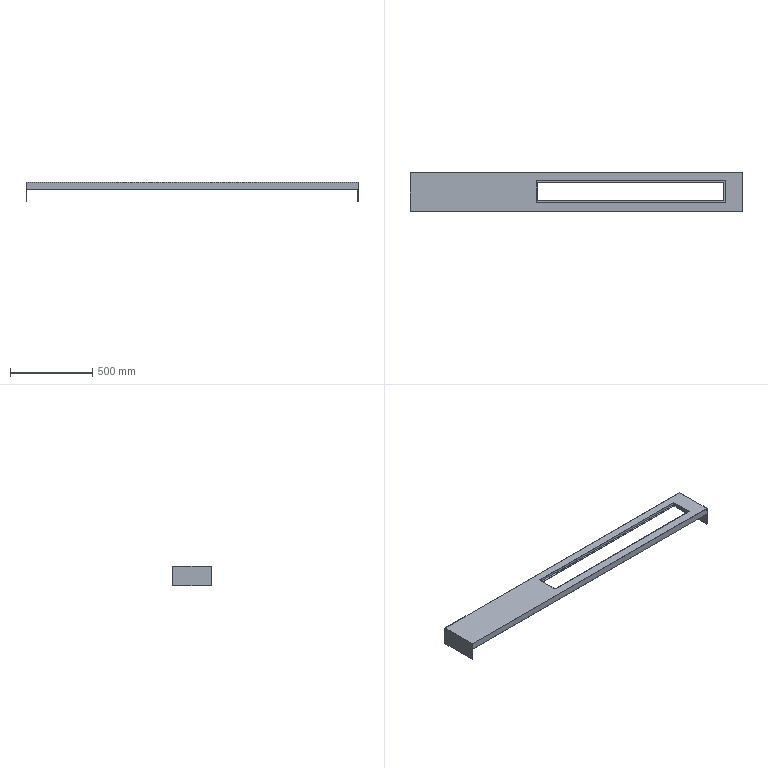Part | SolidWorks | features ICE 6, Extrusion 1 | 1 solid | 28 faces | box 2015 x 235 x 116 mm | volume 1204410 mm3 | plane 28
STEP:
#1=CARTESIAN_POINT('',(1915.,55.,-13.));
#2=VERTEX_POINT('',#1);
#3=CARTESIAN_POINT('',(1915.,185.,-13.));
#4=VERTEX_POINT('',#3);
#5=CARTESIAN_POINT('',(1915.,55.,-13.));
#6=DIRECTION('',(0.,1.,0.));
#7=VECTOR('',#6,1000.);
#8=LINE('',#5,#7);
#9=EDGE_CURVE('',#2,#4,#8,.T.);
#10=ORIENTED_EDGE('',*,*,#9,.F.);
#11=CARTESIAN_POINT('',(1915.,55.,2.));
#12=VERTEX_POINT('',#11);
#13=CARTESIAN_POINT('',(1915.,55.,-8.));
#14=DIRECTION('',(0.,0.,1.));
#15=VECTOR('',#14,1000.);
#16=LINE('',#13,#15);
#17=EDGE_CURVE('',#2,#12,#16,.T.);
#18=ORIENTED_EDGE('',*,*,#17,.T.);
#19=CARTESIAN_POINT('',(1915.,185.,2.));
#20=VERTEX_POINT('',#19);
#21=CARTESIAN_POINT('',(1915.,55.,2.));
#22=DIRECTION('',(0.,1.,0.));
#23=VECTOR('',#22,1000.);
#24=LINE('',#21,#23);
#25=EDGE_CURVE('',#12,#20,#24,.T.);
#26=ORIENTED_EDGE('',*,*,#25,.T.);
#27=CARTESIAN_POINT('',(1915.,185.,-8.));
#28=DIRECTION('',(0.,0.,1.));
#29=VECTOR('',#28,1000.);
#30=LINE('',#27,#29);
#31=EDGE_CURVE('',#4,#20,#30,.T.);
#32=ORIENTED_EDGE('',*,*,#31,.F.);
#33=EDGE_LOOP('',(#10,#18,#26,#32));
#34=FACE_OUTER_BOUND('',#33,.T.);
#35=CARTESIAN_POINT('',(1915.,55.,-8.));
#36=DIRECTION('',(1.,0.,0.));
#37=DIRECTION('',(0.,0.,-1.));
#38=AXIS2_PLACEMENT_3D('',#35,#36,#37);
#39=PLANE('',#38);
#40=ADVANCED_FACE('',(#34),#39,.F.);
#41=CARTESIAN_POINT('',(765.,55.,-13.));
#42=VERTEX_POINT('',#41);
#43=CARTESIAN_POINT('',(1915.,55.,-13.));
#44=DIRECTION('',(1.,0.,0.));
#45=VECTOR('',#44,1000.);
#46=LINE('',#43,#45);
#47=EDGE_CURVE('',#42,#2,#46,.T.);
#48=ORIENTED_EDGE('',*,*,#47,.F.);
#49=CARTESIAN_POINT('',(765.,55.,2.));
#50=VERTEX_POINT('',#49);
#51=CARTESIAN_POINT('',(765.,55.,-8.));
#52=DIRECTION('',(0.,0.,1.));
#53=VECTOR('',#52,1000.);
#54=LINE('',#51,#53);
#55=EDGE_CURVE('',#42,#50,#54,.T.);
#56=ORIENTED_EDGE('',*,*,#55,.T.);
#57=CARTESIAN_POINT('',(1915.,55.,2.));
#58=DIRECTION('',(1.,0.,0.));
#59=VECTOR('',#58,1000.);
#60=LINE('',#57,#59);
#61=EDGE_CURVE('',#50,#12,#60,.T.);
#62=ORIENTED_EDGE('',*,*,#61,.T.);
#63=ORIENTED_EDGE('',*,*,#17,.F.);
#64=EDGE_LOOP('',(#48,#56,#62,#63));
#65=FACE_OUTER_BOUND('',#64,.T.);
#66=CARTESIAN_POINT('',(1915.,55.,-8.));
#67=DIRECTION('',(0.,-1.,0.));
#68=DIRECTION('',(1.,0.,0.));
#69=AXIS2_PLACEMENT_3D('',#66,#67,#68);
#70=PLANE('',#69);
#71=ADVANCED_FACE('',(#65),#70,.F.);
#72=CARTESIAN_POINT('',(765.,185.,-13.));
#73=VERTEX_POINT('',#72);
#74=CARTESIAN_POINT('',(765.,55.,-13.));
#75=DIRECTION('',(0.,-1.,0.));
#76=VECTOR('',#75,1000.);
#77=LINE('',#74,#76);
#78=EDGE_CURVE('',#73,#42,#77,.T.);
#79=ORIENTED_EDGE('',*,*,#78,.F.);
#80=CARTESIAN_POINT('',(765.,185.,2.));
#81=VERTEX_POINT('',#80);
#82=CARTESIAN_POINT('',(765.,185.,-8.));
#83=DIRECTION('',(0.,0.,1.));
#84=VECTOR('',#83,1000.);
#85=LINE('',#82,#84);
#86=EDGE_CURVE('',#73,#81,#85,.T.);
#87=ORIENTED_EDGE('',*,*,#86,.T.);
#88=CARTESIAN_POINT('',(765.,55.,2.));
#89=DIRECTION('',(0.,-1.,0.));
#90=VECTOR('',#89,1000.);
#91=LINE('',#88,#90);
#92=EDGE_CURVE('',#81,#50,#91,.T.);
#93=ORIENTED_EDGE('',*,*,#92,.T.);
#94=ORIENTED_EDGE('',*,*,#55,.F.);
#95=EDGE_LOOP('',(#79,#87,#93,#94));
#96=FACE_OUTER_BOUND('',#95,.T.);
#97=CARTESIAN_POINT('',(765.,55.,-8.));
#98=DIRECTION('',(-1.,0.,0.));
#99=DIRECTION('',(0.,0.,1.));
#100=AXIS2_PLACEMENT_3D('',#97,#98,#99);
#101=PLANE('',#100);
#102=ADVANCED_FACE('',(#96),#101,.F.);
#103=CARTESIAN_POINT('',(1915.,185.,-13.));
#104=DIRECTION('',(-1.,0.,0.));
#105=VECTOR('',#104,1000.);
#106=LINE('',#103,#105);
#107=EDGE_CURVE('',#4,#73,#106,.T.);
#108=ORIENTED_EDGE('',*,*,#107,.F.);
#109=ORIENTED_EDGE('',*,*,#31,.T.);
#110=CARTESIAN_POINT('',(1915.,185.,2.));
#111=DIRECTION('',(-1.,0.,0.));
#112=VECTOR('',#111,1000.);
#113=LINE('',#110,#112);
#114=EDGE_CURVE('',#20,#81,#113,.T.);
#115=ORIENTED_EDGE('',*,*,#114,.T.);
#116=ORIENTED_EDGE('',*,*,#86,.F.);
#117=EDGE_LOOP('',(#108,#109,#115,#116));
#118=FACE_OUTER_BOUND('',#117,.T.);
#119=CARTESIAN_POINT('',(1915.,185.,-8.));
#120=DIRECTION('',(0.,1.,0.));
#121=DIRECTION('',(-1.,0.,0.));
#122=AXIS2_PLACEMENT_3D('',#119,#120,#121);
#123=PLANE('',#122);
#124=ADVANCED_FACE('',(#118),#123,.F.);
#125=CARTESIAN_POINT('',(2013.,2.,0.));
#126=VERTEX_POINT('',#125);
#127=CARTESIAN_POINT('',(2013.,233.,0.));
#128=VERTEX_POINT('',#127);
#129=CARTESIAN_POINT('',(2013.,235.,0.));
#130=DIRECTION('',(0.,1.,0.));
#131=VECTOR('',#130,1000.);
#132=LINE('',#129,#131);
#133=EDGE_CURVE('',#126,#128,#132,.T.);
#134=ORIENTED_EDGE('',*,*,#133,.F.);
#135=CARTESIAN_POINT('',(2.,2.,0.));
#136=VERTEX_POINT('',#135);
#137=CARTESIAN_POINT('',(0.,2.,0.));
#138=DIRECTION('',(-1.,0.,0.));
#139=VECTOR('',#138,1000.);
#140=LINE('',#137,#139);
#141=EDGE_CURVE('',#126,#136,#140,.T.);
#142=ORIENTED_EDGE('',*,*,#141,.T.);
#143=CARTESIAN_POINT('',(2.,233.,0.));
#144=VERTEX_POINT('',#143);
#145=CARTESIAN_POINT('',(2.,235.,0.));
#146=DIRECTION('',(0.,-1.,0.));
#147=VECTOR('',#146,1000.);
#148=LINE('',#145,#147);
#149=EDGE_CURVE('',#144,#136,#148,.T.);
#150=ORIENTED_EDGE('',*,*,#149,.F.);
#151=CARTESIAN_POINT('',(2013.,233.,0.));
#152=DIRECTION('',(-1.,0.,0.));
#153=VECTOR('',#152,1000.);
#154=LINE('',#151,#153);
#155=EDGE_CURVE('',#128,#144,#154,.T.);
#156=ORIENTED_EDGE('',*,*,#155,.F.);
#157=EDGE_LOOP('',(#134,#142,#150,#156));
#158=FACE_OUTER_BOUND('',#157,.T.);
#159=CARTESIAN_POINT('',(1917.,187.,0.));
#160=VERTEX_POINT('',#159);
#161=CARTESIAN_POINT('',(1917.,53.,0.));
#162=VERTEX_POINT('',#161);
#163=CARTESIAN_POINT('',(1917.,187.,0.));
#164=DIRECTION('',(0.,-1.,0.));
#165=VECTOR('',#164,1000.);
#166=LINE('',#163,#165);
#167=EDGE_CURVE('',#160,#162,#166,.T.);
#168=ORIENTED_EDGE('',*,*,#167,.F.);
#169=CARTESIAN_POINT('',(763.,187.,0.));
#170=VERTEX_POINT('',#169);
#171=CARTESIAN_POINT('',(763.,187.,0.));
#172=DIRECTION('',(1.,0.,0.));
#173=VECTOR('',#172,1000.);
#174=LINE('',#171,#173);
#175=EDGE_CURVE('',#170,#160,#174,.T.);
#176=ORIENTED_EDGE('',*,*,#175,.F.);
#177=CARTESIAN_POINT('',(763.,53.,0.));
#178=VERTEX_POINT('',#177);
#179=CARTESIAN_POINT('',(763.,53.,0.));
#180=DIRECTION('',(0.,1.,0.));
#181=VECTOR('',#180,1000.);
#182=LINE('',#179,#181);
#183=EDGE_CURVE('',#178,#170,#182,.T.);
#184=ORIENTED_EDGE('',*,*,#183,.F.);
#185=CARTESIAN_POINT('',(1917.,53.,0.));
#186=DIRECTION('',(-1.,0.,0.));
#187=VECTOR('',#186,1000.);
#188=LINE('',#185,#187);
#189=EDGE_CURVE('',#162,#178,#188,.T.);
#190=ORIENTED_EDGE('',*,*,#189,.F.);
#191=EDGE_LOOP('',(#168,#176,#184,#190));
#192=FACE_BOUND('',#191,.T.);
#193=CARTESIAN_POINT('',(0.,235.,0.));
#194=DIRECTION('',(0.,0.,-1.));
#195=DIRECTION('',(-1.,0.,0.));
#196=AXIS2_PLACEMENT_3D('',#193,#194,#195);
#197=PLANE('',#196);
#198=ADVANCED_FACE('',(#158,#192),#197,.T.);
#199=CARTESIAN_POINT('',(2013.,0.,-114.));
#200=VERTEX_POINT('',#199);
#201=CARTESIAN_POINT('',(2013.,0.,-40.));
#202=VERTEX_POINT('',#201);
#203=CARTESIAN_POINT('',(2013.,0.,-114.));
#204=DIRECTION('',(0.,0.,1.));
#205=VECTOR('',#204,1000.);
#206=LINE('',#203,#205);
#207=EDGE_CURVE('',#200,#202,#206,.T.);
#208=ORIENTED_EDGE('',*,*,#207,.T.);
#209=CARTESIAN_POINT('',(2013.,2.,-40.));
#210=VERTEX_POINT('',#209);
#211=CARTESIAN_POINT('',(2013.,235.,-40.));
#212=DIRECTION('',(0.,1.,0.));
#213=VECTOR('',#212,1000.);
#214=LINE('',#211,#213);
#215=EDGE_CURVE('',#202,#210,#214,.T.);
#216=ORIENTED_EDGE('',*,*,#215,.T.);
#217=CARTESIAN_POINT('',(2013.,2.,-114.));
#218=DIRECTION('',(0.,0.,-1.));
#219=VECTOR('',#218,1000.);
#220=LINE('',#217,#219);
#221=EDGE_CURVE('',#126,#210,#220,.T.);
#222=ORIENTED_EDGE('',*,*,#221,.F.);
#223=ORIENTED_EDGE('',*,*,#133,.T.);
#224=CARTESIAN_POINT('',(2013.,233.,-40.));
#225=VERTEX_POINT('',#224);
#226=CARTESIAN_POINT('',(2013.,233.,-40.));
#227=DIRECTION('',(0.,0.,1.));
#228=VECTOR('',#227,1000.);
#229=LINE('',#226,#228);
#230=EDGE_CURVE('',#225,#128,#229,.T.);
#231=ORIENTED_EDGE('',*,*,#230,.F.);
#232=CARTESIAN_POINT('',(2013.,235.,-40.));
#233=VERTEX_POINT('',#232);
#234=CARTESIAN_POINT('',(2013.,235.,-40.));
#235=DIRECTION('',(0.,-1.,0.));
#236=VECTOR('',#235,1000.);
#237=LINE('',#234,#236);
#238=EDGE_CURVE('',#233,#225,#237,.T.);
#239=ORIENTED_EDGE('',*,*,#238,.F.);
#240=CARTESIAN_POINT('',(2013.,235.,-114.));
#241=VERTEX_POINT('',#240);
#242=CARTESIAN_POINT('',(2013.,235.,-114.));
#243=DIRECTION('',(0.,0.,1.));
#244=VECTOR('',#243,1000.);
#245=LINE('',#242,#244);
#246=EDGE_CURVE('',#241,#233,#245,.T.);
#247=ORIENTED_EDGE('',*,*,#246,.F.);
#248=CARTESIAN_POINT('',(2013.,235.,-114.));
#249=DIRECTION('',(0.,1.,0.));
#250=VECTOR('',#249,1000.);
#251=LINE('',#248,#250);
#252=EDGE_CURVE('',#200,#241,#251,.T.);
#253=ORIENTED_EDGE('',*,*,#252,.F.);
#254=EDGE_LOOP('',(#208,#216,#222,#223,#231,#239,#247,#253));
#255=FACE_OUTER_BOUND('',#254,.T.);
#256=CARTESIAN_POINT('',(2013.,235.,-114.));
#257=DIRECTION('',(1.,0.,0.));
#258=DIRECTION('',(0.,0.,-1.));
#259=AXIS2_PLACEMENT_3D('',#256,#257,#258);
#260=PLANE('',#259);
#261=ADVANCED_FACE('',(#255),#260,.F.);
#262=CARTESIAN_POINT('',(2.,2.,-40.));
#263=VERTEX_POINT('',#262);
#264=CARTESIAN_POINT('',(2.,2.,-114.));
#265=DIRECTION('',(0.,0.,1.));
#266=VECTOR('',#265,1000.);
#267=LINE('',#264,#266);
#268=EDGE_CURVE('',#263,#136,#267,.T.);
#269=ORIENTED_EDGE('',*,*,#268,.F.);
#270=CARTESIAN_POINT('',(2.,0.,-40.));
#271=VERTEX_POINT('',#270);
#272=CARTESIAN_POINT('',(2.,235.,-40.));
#273=DIRECTION('',(0.,-1.,0.));
#274=VECTOR('',#273,1000.);
#275=LINE('',#272,#274);
#276=EDGE_CURVE('',#263,#271,#275,.T.);
#277=ORIENTED_EDGE('',*,*,#276,.T.);
#278=CARTESIAN_POINT('',(2.,0.,-114.));
#279=VERTEX_POINT('',#278);
#280=CARTESIAN_POINT('',(2.,0.,-114.));
#281=DIRECTION('',(0.,0.,1.));
#282=VECTOR('',#281,1000.);
#283=LINE('',#280,#282);
#284=EDGE_CURVE('',#279,#271,#283,.T.);
#285=ORIENTED_EDGE('',*,*,#284,.F.);
#286=CARTESIAN_POINT('',(2.,235.,-114.));
#287=VERTEX_POINT('',#286);
#288=CARTESIAN_POINT('',(2.,235.,-114.));
#289=DIRECTION('',(0.,-1.,0.));
#290=VECTOR('',#289,1000.);
#291=LINE('',#288,#290);
#292=EDGE_CURVE('',#287,#279,#291,.T.);
#293=ORIENTED_EDGE('',*,*,#292,.F.);
#294=CARTESIAN_POINT('',(2.,235.,-40.));
#295=VERTEX_POINT('',#294);
#296=CARTESIAN_POINT('',(2.,235.,-114.));
#297=DIRECTION('',(0.,0.,1.));
#298=VECTOR('',#297,1000.);
#299=LINE('',#296,#298);
#300=EDGE_CURVE('',#287,#295,#299,.T.);
#301=ORIENTED_EDGE('',*,*,#300,.T.);
#302=CARTESIAN_POINT('',(2.,233.,-40.));
#303=VERTEX_POINT('',#302);
#304=CARTESIAN_POINT('',(2.,235.,-40.));
#305=DIRECTION('',(0.,1.,0.));
#306=VECTOR('',#305,1000.);
#307=LINE('',#304,#306);
#308=EDGE_CURVE('',#303,#295,#307,.T.);
#309=ORIENTED_EDGE('',*,*,#308,.F.);
#310=CARTESIAN_POINT('',(2.,233.,-40.));
#311=DIRECTION('',(0.,0.,1.));
#312=VECTOR('',#311,1000.);
#313=LINE('',#310,#312);
#314=EDGE_CURVE('',#303,#144,#313,.T.);
#315=ORIENTED_EDGE('',*,*,#314,.T.);
#316=ORIENTED_EDGE('',*,*,#149,.T.);
#317=EDGE_LOOP('',(#269,#277,#285,#293,#301,#309,#315,#316));
#318=FACE_OUTER_BOUND('',#317,.T.);
#319=CARTESIAN_POINT('',(2.,235.,-114.));
#320=DIRECTION('',(-1.,0.,0.));
#321=DIRECTION('',(0.,0.,1.));
#322=AXIS2_PLACEMENT_3D('',#319,#320,#321);
#323=PLANE('',#322);
#324=ADVANCED_FACE('',(#318),#323,.F.);
#325=CARTESIAN_POINT('',(0.,0.,-114.));
#326=VERTEX_POINT('',#325);
#327=CARTESIAN_POINT('',(0.,235.,-114.));
#328=VERTEX_POINT('',#327);
#329=CARTESIAN_POINT('',(0.,235.,-114.));
#330=DIRECTION('',(0.,1.,0.));
#331=VECTOR('',#330,1000.);
#332=LINE('',#329,#331);
#333=EDGE_CURVE('',#326,#328,#332,.T.);
#334=ORIENTED_EDGE('',*,*,#333,.F.);
#335=CARTESIAN_POINT('',(0.,0.,2.));
#336=VERTEX_POINT('',#335);
#337=CARTESIAN_POINT('',(0.,0.,2.));
#338=DIRECTION('',(0.,0.,-1.));
#339=VECTOR('',#338,1000.);
#340=LINE('',#337,#339);
#341=EDGE_CURVE('',#336,#326,#340,.T.);
#342=ORIENTED_EDGE('',*,*,#341,.F.);
#343=CARTESIAN_POINT('',(0.,235.,2.));
#344=VERTEX_POINT('',#343);
#345=CARTESIAN_POINT('',(0.,0.,2.));
#346=DIRECTION('',(0.,-1.,0.));
#347=VECTOR('',#346,1000.);
#348=LINE('',#345,#347);
#349=EDGE_CURVE('',#344,#336,#348,.T.);
#350=ORIENTED_EDGE('',*,*,#349,.F.);
#351=CARTESIAN_POINT('',(0.,235.,2.));
#352=DIRECTION('',(0.,0.,-1.));
#353=VECTOR('',#352,1000.);
#354=LINE('',#351,#353);
#355=EDGE_CURVE('',#344,#328,#354,.T.);
#356=ORIENTED_EDGE('',*,*,#355,.T.);
#357=EDGE_LOOP('',(#334,#342,#350,#356));
#358=FACE_OUTER_BOUND('',#357,.T.);
#359=CARTESIAN_POINT('',(0.,0.,2.));
#360=DIRECTION('',(1.,0.,0.));
#361=DIRECTION('',(0.,0.,-1.));
#362=AXIS2_PLACEMENT_3D('',#359,#360,#361);
#363=PLANE('',#362);
#364=ADVANCED_FACE('',(#358),#363,.F.);
#365=CARTESIAN_POINT('',(0.,0.,-40.));
#366=DIRECTION('',(1.,0.,0.));
#367=VECTOR('',#366,1000.);
#368=LINE('',#365,#367);
#369=EDGE_CURVE('',#271,#202,#368,.T.);
#370=ORIENTED_EDGE('',*,*,#369,.T.);
#371=ORIENTED_EDGE('',*,*,#207,.F.);
#372=CARTESIAN_POINT('',(2015.,0.,-114.));
#373=VERTEX_POINT('',#372);
#374=CARTESIAN_POINT('',(2015.,0.,-114.));
#375=DIRECTION('',(-1.,0.,0.));
#376=VECTOR('',#375,1000.);
#377=LINE('',#374,#376);
#378=EDGE_CURVE('',#373,#200,#377,.T.);
#379=ORIENTED_EDGE('',*,*,#378,.F.);
#380=CARTESIAN_POINT('',(2015.,0.,2.));
#381=VERTEX_POINT('',#380);
#382=CARTESIAN_POINT('',(2015.,0.,2.));
#383=DIRECTION('',(0.,0.,-1.));
#384=VECTOR('',#383,1000.);
#385=LINE('',#382,#384);
#386=EDGE_CURVE('',#381,#373,#385,.T.);
#387=ORIENTED_EDGE('',*,*,#386,.F.);
#388=CARTESIAN_POINT('',(0.,0.,2.));
#389=DIRECTION('',(1.,0.,0.));
#390=VECTOR('',#389,1000.);
#391=LINE('',#388,#390);
#392=EDGE_CURVE('',#336,#381,#391,.T.);
#393=ORIENTED_EDGE('',*,*,#392,.F.);
#394=ORIENTED_EDGE('',*,*,#341,.T.);
#395=CARTESIAN_POINT('',(0.,0.,-114.));
#396=DIRECTION('',(-1.,0.,0.));
#397=VECTOR('',#396,1000.);
#398=LINE('',#395,#397);
#399=EDGE_CURVE('',#279,#326,#398,.T.);
#400=ORIENTED_EDGE('',*,*,#399,.F.);
#401=ORIENTED_EDGE('',*,*,#284,.T.);
#402=EDGE_LOOP('',(#370,#371,#379,#387,#393,#394,#400,#401));
#403=FACE_OUTER_BOUND('',#402,.T.);
#404=CARTESIAN_POINT('',(0.,0.,2.));
#405=DIRECTION('',(0.,1.,0.));
#406=DIRECTION('',(0.,0.,1.));
#407=AXIS2_PLACEMENT_3D('',#404,#405,#406);
#408=PLANE('',#407);
#409=ADVANCED_FACE('',(#403),#408,.F.);
#410=ORIENTED_EDGE('',*,*,#386,.T.);
#411=CARTESIAN_POINT('',(2015.,235.,-114.));
#412=VERTEX_POINT('',#411);
#413=CARTESIAN_POINT('',(2015.,235.,-114.));
#414=DIRECTION('',(0.,-1.,0.));
#415=VECTOR('',#414,1000.);
#416=LINE('',#413,#415);
#417=EDGE_CURVE('',#412,#373,#416,.T.);
#418=ORIENTED_EDGE('',*,*,#417,.F.);
#419=CARTESIAN_POINT('',(2015.,235.,2.));
#420=VERTEX_POINT('',#419);
#421=CARTESIAN_POINT('',(2015.,235.,2.));
#422=DIRECTION('',(0.,0.,-1.));
#423=VECTOR('',#422,1000.);
#424=LINE('',#421,#423);
#425=EDGE_CURVE('',#420,#412,#424,.T.);
#426=ORIENTED_EDGE('',*,*,#425,.F.);
#427=CARTESIAN_POINT('',(2015.,0.,2.));
#428=DIRECTION('',(0.,1.,0.));
#429=VECTOR('',#428,1000.);
#430=LINE('',#427,#429);
#431=EDGE_CURVE('',#381,#420,#430,.T.);
#432=ORIENTED_EDGE('',*,*,#431,.F.);
#433=EDGE_LOOP('',(#410,#418,#426,#432));
#434=FACE_OUTER_BOUND('',#433,.T.);
#435=CARTESIAN_POINT('',(2015.,0.,2.));
#436=DIRECTION('',(-1.,0.,0.));
#437=DIRECTION('',(0.,0.,1.));
#438=AXIS2_PLACEMENT_3D('',#435,#436,#437);
#439=PLANE('',#438);
#440=ADVANCED_FACE('',(#434),#439,.F.);
#441=ORIENTED_EDGE('',*,*,#425,.T.);
#442=CARTESIAN_POINT('',(2015.,235.,-114.));
#443=DIRECTION('',(1.,0.,0.));
#444=VECTOR('',#443,1000.);
#445=LINE('',#442,#444);
#446=EDGE_CURVE('',#241,#412,#445,.T.);
#447=ORIENTED_EDGE('',*,*,#446,.F.);
#448=ORIENTED_EDGE('',*,*,#246,.T.);
#449=CARTESIAN_POINT('',(2013.,235.,-40.));
#450=DIRECTION('',(1.,0.,0.));
#451=VECTOR('',#450,1000.);
#452=LINE('',#449,#451);
#453=EDGE_CURVE('',#295,#233,#452,.T.);
#454=ORIENTED_EDGE('',*,*,#453,.F.);
#455=ORIENTED_EDGE('',*,*,#300,.F.);
#456=CARTESIAN_POINT('',(0.,235.,-114.));
#457=DIRECTION('',(1.,0.,0.));
#458=VECTOR('',#457,1000.);
#459=LINE('',#456,#458);
#460=EDGE_CURVE('',#328,#287,#459,.T.);
#461=ORIENTED_EDGE('',*,*,#460,.F.);
#462=ORIENTED_EDGE('',*,*,#355,.F.);
#463=CARTESIAN_POINT('',(0.,235.,2.));
#464=DIRECTION('',(-1.,0.,0.));
#465=VECTOR('',#464,1000.);
#466=LINE('',#463,#465);
#467=EDGE_CURVE('',#420,#344,#466,.T.);
#468=ORIENTED_EDGE('',*,*,#467,.F.);
#469=EDGE_LOOP('',(#441,#447,#448,#454,#455,#461,#462,#468));
#470=FACE_OUTER_BOUND('',#469,.T.);
#471=CARTESIAN_POINT('',(0.,235.,2.));
#472=DIRECTION('',(0.,-1.,0.));
#473=DIRECTION('',(0.,0.,-1.));
#474=AXIS2_PLACEMENT_3D('',#471,#472,#473);
#475=PLANE('',#474);
#476=ADVANCED_FACE('',(#470),#475,.F.);
#477=ORIENTED_EDGE('',*,*,#431,.T.);
#478=ORIENTED_EDGE('',*,*,#467,.T.);
#479=ORIENTED_EDGE('',*,*,#349,.T.);
#480=ORIENTED_EDGE('',*,*,#392,.T.);
#481=EDGE_LOOP('',(#477,#478,#479,#480));
#482=FACE_OUTER_BOUND('',#481,.T.);
#483=ORIENTED_EDGE('',*,*,#114,.F.);
#484=ORIENTED_EDGE('',*,*,#25,.F.);
#485=ORIENTED_EDGE('',*,*,#61,.F.);
#486=ORIENTED_EDGE('',*,*,#92,.F.);
#487=EDGE_LOOP('',(#483,#484,#485,#486));
#488=FACE_BOUND('',#487,.T.);
#489=CARTESIAN_POINT('',(0.,235.,2.));
#490=DIRECTION('',(0.,0.,-1.));
#491=DIRECTION('',(-1.,0.,0.));
#492=AXIS2_PLACEMENT_3D('',#489,#490,#491);
#493=PLANE('',#492);
#494=ADVANCED_FACE('',(#482,#488),#493,.F.);
#495=ORIENTED_EDGE('',*,*,#417,.T.);
#496=ORIENTED_EDGE('',*,*,#378,.T.);
#497=ORIENTED_EDGE('',*,*,#252,.T.);
#498=ORIENTED_EDGE('',*,*,#446,.T.);
#499=EDGE_LOOP('',(#495,#496,#497,#498));
#500=FACE_OUTER_BOUND('',#499,.T.);
#501=CARTESIAN_POINT('',(2015.,0.,-114.));
#502=DIRECTION('',(0.,0.,-1.));
#503=DIRECTION('',(-1.,0.,0.));
#504=AXIS2_PLACEMENT_3D('',#501,#502,#503);
#505=PLANE('',#504);
#506=ADVANCED_FACE('',(#500),#505,.T.);
#507=ORIENTED_EDGE('',*,*,#460,.T.);
#508=ORIENTED_EDGE('',*,*,#292,.T.);
#509=ORIENTED_EDGE('',*,*,#399,.T.);
#510=ORIENTED_EDGE('',*,*,#333,.T.);
#511=EDGE_LOOP('',(#507,#508,#509,#510));
#512=FACE_OUTER_BOUND('',#511,.T.);
#513=CARTESIAN_POINT('',(2.,235.,-114.));
#514=DIRECTION('',(0.,0.,-1.));
#515=DIRECTION('',(-1.,0.,0.));
#516=AXIS2_PLACEMENT_3D('',#513,#514,#515);
#517=PLANE('',#516);
#518=ADVANCED_FACE('',(#512),#517,.T.);
#519=ORIENTED_EDGE('',*,*,#155,.T.);
#520=ORIENTED_EDGE('',*,*,#314,.F.);
#521=CARTESIAN_POINT('',(2013.,233.,-40.));
#522=DIRECTION('',(-1.,0.,0.));
#523=VECTOR('',#522,1000.);
#524=LINE('',#521,#523);
#525=EDGE_CURVE('',#225,#303,#524,.T.);
#526=ORIENTED_EDGE('',*,*,#525,.F.);
#527=ORIENTED_EDGE('',*,*,#230,.T.);
#528=EDGE_LOOP('',(#519,#520,#526,#527));
#529=FACE_OUTER_BOUND('',#528,.T.);
#530=CARTESIAN_POINT('',(2013.,233.,-40.));
#531=DIRECTION('',(0.,1.,0.));
#532=DIRECTION('',(0.,0.,1.));
#533=AXIS2_PLACEMENT_3D('',#530,#531,#532);
#534=PLANE('',#533);
#535=ADVANCED_FACE('',(#529),#534,.F.);
#536=ORIENTED_EDGE('',*,*,#238,.T.);
#537=ORIENTED_EDGE('',*,*,#525,.T.);
#538=ORIENTED_EDGE('',*,*,#308,.T.);
#539=ORIENTED_EDGE('',*,*,#453,.T.);
#540=EDGE_LOOP('',(#536,#537,#538,#539));
#541=FACE_OUTER_BOUND('',#540,.T.);
#542=CARTESIAN_POINT('',(2013.,233.,-40.));
#543=DIRECTION('',(0.,0.,-1.));
#544=DIRECTION('',(-1.,0.,0.));
#545=AXIS2_PLACEMENT_3D('',#542,#543,#544);
#546=PLANE('',#545);
#547=ADVANCED_FACE('',(#541),#546,.T.);
#548=ORIENTED_EDGE('',*,*,#215,.F.);
#549=ORIENTED_EDGE('',*,*,#369,.F.);
#550=ORIENTED_EDGE('',*,*,#276,.F.);
#551=CARTESIAN_POINT('',(0.,2.,-40.));
#552=DIRECTION('',(1.,0.,0.));
#553=VECTOR('',#552,1000.);
#554=LINE('',#551,#553);
#555=EDGE_CURVE('',#263,#210,#554,.T.);
#556=ORIENTED_EDGE('',*,*,#555,.T.);
#557=EDGE_LOOP('',(#548,#549,#550,#556));
#558=FACE_OUTER_BOUND('',#557,.T.);
#559=CARTESIAN_POINT('',(0.,2.,-40.));
#560=DIRECTION('',(0.,0.,-1.));
#561=DIRECTION('',(-1.,0.,0.));
#562=AXIS2_PLACEMENT_3D('',#559,#560,#561);
#563=PLANE('',#562);
#564=ADVANCED_FACE('',(#558),#563,.T.);
#565=ORIENTED_EDGE('',*,*,#141,.F.);
#566=ORIENTED_EDGE('',*,*,#221,.T.);
#567=ORIENTED_EDGE('',*,*,#555,.F.);
#568=ORIENTED_EDGE('',*,*,#268,.T.);
#569=EDGE_LOOP('',(#565,#566,#567,#568));
#570=FACE_OUTER_BOUND('',#569,.T.);
#571=CARTESIAN_POINT('',(0.,2.,-40.));
#572=DIRECTION('',(0.,-1.,0.));
#573=DIRECTION('',(0.,0.,-1.));
#574=AXIS2_PLACEMENT_3D('',#571,#572,#573);
#575=PLANE('',#574);
#576=ADVANCED_FACE('',(#570),#575,.F.);
#577=CARTESIAN_POINT('',(763.,187.,-15.));
#578=VERTEX_POINT('',#577);
#579=CARTESIAN_POINT('',(1917.,187.,-15.));
#580=VERTEX_POINT('',#579);
#581=CARTESIAN_POINT('',(763.,187.,-15.));
#582=DIRECTION('',(1.,0.,0.));
#583=VECTOR('',#582,1000.);
#584=LINE('',#581,#583);
#585=EDGE_CURVE('',#578,#580,#584,.T.);
#586=ORIENTED_EDGE('',*,*,#585,.T.);
#587=CARTESIAN_POINT('',(1917.,53.,-15.));
#588=VERTEX_POINT('',#587);
#589=CARTESIAN_POINT('',(1917.,187.,-15.));
#590=DIRECTION('',(0.,-1.,0.));
#591=VECTOR('',#590,1000.);
#592=LINE('',#589,#591);
#593=EDGE_CURVE('',#580,#588,#592,.T.);
#594=ORIENTED_EDGE('',*,*,#593,.T.);
#595=CARTESIAN_POINT('',(763.,53.,-15.));
#596=VERTEX_POINT('',#595);
#597=CARTESIAN_POINT('',(1917.,53.,-15.));
#598=DIRECTION('',(-1.,0.,0.));
#599=VECTOR('',#598,1000.);
#600=LINE('',#597,#599);
#601=EDGE_CURVE('',#588,#596,#600,.T.);
#602=ORIENTED_EDGE('',*,*,#601,.T.);
#603=CARTESIAN_POINT('',(763.,53.,-15.));
#604=DIRECTION('',(0.,1.,0.));
#605=VECTOR('',#604,1000.);
#606=LINE('',#603,#605);
#607=EDGE_CURVE('',#596,#578,#606,.T.);
#608=ORIENTED_EDGE('',*,*,#607,.T.);
#609=EDGE_LOOP('',(#586,#594,#602,#608));
#610=FACE_OUTER_BOUND('',#609,.T.);
#611=CARTESIAN_POINT('',(775.,175.,-15.));
#612=VERTEX_POINT('',#611);
#613=CARTESIAN_POINT('',(1905.,175.,-15.));
#614=VERTEX_POINT('',#613);
#615=CARTESIAN_POINT('',(775.,175.,-15.));
#616=DIRECTION('',(1.,0.,0.));
#617=VECTOR('',#616,1000.);
#618=LINE('',#615,#617);
#619=EDGE_CURVE('',#612,#614,#618,.T.);
#620=ORIENTED_EDGE('',*,*,#619,.F.);
#621=CARTESIAN_POINT('',(775.,65.,-15.));
#622=VERTEX_POINT('',#621);
#623=CARTESIAN_POINT('',(775.,65.,-15.));
#624=DIRECTION('',(0.,1.,0.));
#625=VECTOR('',#624,1000.);
#626=LINE('',#623,#625);
#627=EDGE_CURVE('',#622,#612,#626,.T.);
#628=ORIENTED_EDGE('',*,*,#627,.F.);
#629=CARTESIAN_POINT('',(1905.,65.,-15.));
#630=VERTEX_POINT('',#629);
#631=CARTESIAN_POINT('',(1905.,65.,-15.));
#632=DIRECTION('',(-1.,0.,0.));
#633=VECTOR('',#632,1000.);
#634=LINE('',#631,#633);
#635=EDGE_CURVE('',#630,#622,#634,.T.);
#636=ORIENTED_EDGE('',*,*,#635,.F.);
#637=CARTESIAN_POINT('',(1905.,175.,-15.));
#638=DIRECTION('',(0.,-1.,0.));
#639=VECTOR('',#638,1000.);
#640=LINE('',#637,#639);
#641=EDGE_CURVE('',#614,#630,#640,.T.);
#642=ORIENTED_EDGE('',*,*,#641,.F.);
#643=EDGE_LOOP('',(#620,#628,#636,#642));
#644=FACE_BOUND('',#643,.T.);
#645=CARTESIAN_POINT('',(1917.,187.,-15.));
#646=DIRECTION('',(0.,0.,-1.));
#647=DIRECTION('',(-1.,0.,0.));
#648=AXIS2_PLACEMENT_3D('',#645,#646,#647);
#649=PLANE('',#648);
#650=ADVANCED_FACE('',(#610,#644),#649,.T.);
#651=CARTESIAN_POINT('',(763.,187.,-15.));
#652=DIRECTION('',(0.,0.,1.));
#653=VECTOR('',#652,1000.);
#654=LINE('',#651,#653);
#655=EDGE_CURVE('',#578,#170,#654,.T.);
#656=ORIENTED_EDGE('',*,*,#655,.T.);
#657=ORIENTED_EDGE('',*,*,#175,.T.);
#658=CARTESIAN_POINT('',(1917.,187.,-15.));
#659=DIRECTION('',(0.,0.,1.));
#660=VECTOR('',#659,1000.);
#661=LINE('',#658,#660);
#662=EDGE_CURVE('',#580,#160,#661,.T.);
#663=ORIENTED_EDGE('',*,*,#662,.F.);
#664=ORIENTED_EDGE('',*,*,#585,.F.);
#665=EDGE_LOOP('',(#656,#657,#663,#664));
#666=FACE_OUTER_BOUND('',#665,.T.);
#667=CARTESIAN_POINT('',(763.,187.,-15.));
#668=DIRECTION('',(0.,-1.,0.));
#669=DIRECTION('',(1.,0.,0.));
#670=AXIS2_PLACEMENT_3D('',#667,#668,#669);
#671=PLANE('',#670);
#672=ADVANCED_FACE('',(#666),#671,.F.);
#673=ORIENTED_EDGE('',*,*,#662,.T.);
#674=ORIENTED_EDGE('',*,*,#167,.T.);
#675=CARTESIAN_POINT('',(1917.,53.,-15.));
#676=DIRECTION('',(0.,0.,1.));
#677=VECTOR('',#676,1000.);
#678=LINE('',#675,#677);
#679=EDGE_CURVE('',#588,#162,#678,.T.);
#680=ORIENTED_EDGE('',*,*,#679,.F.);
#681=ORIENTED_EDGE('',*,*,#593,.F.);
#682=EDGE_LOOP('',(#673,#674,#680,#681));
#683=FACE_OUTER_BOUND('',#682,.T.);
#684=CARTESIAN_POINT('',(1917.,187.,-15.));
#685=DIRECTION('',(-1.,0.,0.));
#686=DIRECTION('',(0.,0.,1.));
#687=AXIS2_PLACEMENT_3D('',#684,#685,#686);
#688=PLANE('',#687);
#689=ADVANCED_FACE('',(#683),#688,.F.);
#690=ORIENTED_EDGE('',*,*,#679,.T.);
#691=ORIENTED_EDGE('',*,*,#189,.T.);
#692=CARTESIAN_POINT('',(763.,53.,-15.));
#693=DIRECTION('',(0.,0.,1.));
#694=VECTOR('',#693,1000.);
#695=LINE('',#692,#694);
#696=EDGE_CURVE('',#596,#178,#695,.T.);
#697=ORIENTED_EDGE('',*,*,#696,.F.);
#698=ORIENTED_EDGE('',*,*,#601,.F.);
#699=EDGE_LOOP('',(#690,#691,#697,#698));
#700=FACE_OUTER_BOUND('',#699,.T.);
#701=CARTESIAN_POINT('',(1917.,53.,-15.));
#702=DIRECTION('',(0.,1.,0.));
#703=DIRECTION('',(-1.,0.,0.));
#704=AXIS2_PLACEMENT_3D('',#701,#702,#703);
#705=PLANE('',#704);
#706=ADVANCED_FACE('',(#700),#705,.F.);
#707=ORIENTED_EDGE('',*,*,#696,.T.);
#708=ORIENTED_EDGE('',*,*,#183,.T.);
#709=ORIENTED_EDGE('',*,*,#655,.F.);
#710=ORIENTED_EDGE('',*,*,#607,.F.);
#711=EDGE_LOOP('',(#707,#708,#709,#710));
#712=FACE_OUTER_BOUND('',#711,.T.);
#713=CARTESIAN_POINT('',(763.,53.,-15.));
#714=DIRECTION('',(1.,0.,0.));
#715=DIRECTION('',(0.,0.,-1.));
#716=AXIS2_PLACEMENT_3D('',#713,#714,#715);
#717=PLANE('',#716);
#718=ADVANCED_FACE('',(#712),#717,.F.);
#719=CARTESIAN_POINT('',(775.,65.,-13.));
#720=VERTEX_POINT('',#719);
#721=CARTESIAN_POINT('',(775.,175.,-13.));
#722=VERTEX_POINT('',#721);
#723=CARTESIAN_POINT('',(775.,65.,-13.));
#724=DIRECTION('',(0.,1.,0.));
#725=VECTOR('',#724,1000.);
#726=LINE('',#723,#725);
#727=EDGE_CURVE('',#720,#722,#726,.T.);
#728=ORIENTED_EDGE('',*,*,#727,.T.);
#729=CARTESIAN_POINT('',(1905.,175.,-13.));
#730=VERTEX_POINT('',#729);
#731=CARTESIAN_POINT('',(775.,175.,-13.));
#732=DIRECTION('',(1.,0.,0.));
#733=VECTOR('',#732,1000.);
#734=LINE('',#731,#733);
#735=EDGE_CURVE('',#722,#730,#734,.T.);
#736=ORIENTED_EDGE('',*,*,#735,.T.);
#737=CARTESIAN_POINT('',(1905.,65.,-13.));
#738=VERTEX_POINT('',#737);
#739=CARTESIAN_POINT('',(1905.,175.,-13.));
#740=DIRECTION('',(0.,-1.,0.));
#741=VECTOR('',#740,1000.);
#742=LINE('',#739,#741);
#743=EDGE_CURVE('',#730,#738,#742,.T.);
#744=ORIENTED_EDGE('',*,*,#743,.T.);
#745=CARTESIAN_POINT('',(1905.,65.,-13.));
#746=DIRECTION('',(-1.,0.,0.));
#747=VECTOR('',#746,1000.);
#748=LINE('',#745,#747);
#749=EDGE_CURVE('',#738,#720,#748,.T.);
#750=ORIENTED_EDGE('',*,*,#749,.T.);
#751=EDGE_LOOP('',(#728,#736,#744,#750));
#752=FACE_BOUND('',#751,.T.);
#753=ORIENTED_EDGE('',*,*,#47,.T.);
#754=ORIENTED_EDGE('',*,*,#9,.T.);
#755=ORIENTED_EDGE('',*,*,#107,.T.);
#756=ORIENTED_EDGE('',*,*,#78,.T.);
#757=EDGE_LOOP('',(#753,#754,#755,#756));
#758=FACE_OUTER_BOUND('',#757,.T.);
#759=CARTESIAN_POINT('',(1917.,53.,-13.));
#760=DIRECTION('',(0.,0.,-1.));
#761=DIRECTION('',(-1.,0.,0.));
#762=AXIS2_PLACEMENT_3D('',#759,#760,#761);
#763=PLANE('',#762);
#764=ADVANCED_FACE('',(#752,#758),#763,.F.);
#765=ORIENTED_EDGE('',*,*,#619,.T.);
#766=CARTESIAN_POINT('',(1905.,175.,-13.));
#767=DIRECTION('',(0.,0.,-1.));
#768=VECTOR('',#767,1000.);
#769=LINE('',#766,#768);
#770=EDGE_CURVE('',#730,#614,#769,.T.);
#771=ORIENTED_EDGE('',*,*,#770,.F.);
#772=ORIENTED_EDGE('',*,*,#735,.F.);
#773=CARTESIAN_POINT('',(775.,175.,-13.));
#774=DIRECTION('',(0.,0.,-1.));
#775=VECTOR('',#774,1000.);
#776=LINE('',#773,#775);
#777=EDGE_CURVE('',#722,#612,#776,.T.);
#778=ORIENTED_EDGE('',*,*,#777,.T.);
#779=EDGE_LOOP('',(#765,#771,#772,#778));
#780=FACE_OUTER_BOUND('',#779,.T.);
#781=CARTESIAN_POINT('',(775.,175.,-13.));
#782=DIRECTION('',(0.,1.,0.));
#783=DIRECTION('',(-1.,0.,0.));
#784=AXIS2_PLACEMENT_3D('',#781,#782,#783);
#785=PLANE('',#784);
#786=ADVANCED_FACE('',(#780),#785,.F.);
#787=ORIENTED_EDGE('',*,*,#627,.T.);
#788=ORIENTED_EDGE('',*,*,#777,.F.);
#789=ORIENTED_EDGE('',*,*,#727,.F.);
#790=CARTESIAN_POINT('',(775.,65.,-13.));
#791=DIRECTION('',(0.,0.,-1.));
#792=VECTOR('',#791,1000.);
#793=LINE('',#790,#792);
#794=EDGE_CURVE('',#720,#622,#793,.T.);
#795=ORIENTED_EDGE('',*,*,#794,.T.);
#796=EDGE_LOOP('',(#787,#788,#789,#795));
#797=FACE_OUTER_BOUND('',#796,.T.);
#798=CARTESIAN_POINT('',(775.,65.,-13.));
#799=DIRECTION('',(-1.,0.,0.));
#800=DIRECTION('',(0.,0.,1.));
#801=AXIS2_PLACEMENT_3D('',#798,#799,#800);
#802=PLANE('',#801);
#803=ADVANCED_FACE('',(#797),#802,.F.);
#804=ORIENTED_EDGE('',*,*,#635,.T.);
#805=ORIENTED_EDGE('',*,*,#794,.F.);
#806=ORIENTED_EDGE('',*,*,#749,.F.);
#807=CARTESIAN_POINT('',(1905.,65.,-13.));
#808=DIRECTION('',(0.,0.,-1.));
#809=VECTOR('',#808,1000.);
#810=LINE('',#807,#809);
#811=EDGE_CURVE('',#738,#630,#810,.T.);
#812=ORIENTED_EDGE('',*,*,#811,.T.);
#813=EDGE_LOOP('',(#804,#805,#806,#812));
#814=FACE_OUTER_BOUND('',#813,.T.);
#815=CARTESIAN_POINT('',(1905.,65.,-13.));
#816=DIRECTION('',(0.,-1.,0.));
#817=DIRECTION('',(1.,0.,0.));
#818=AXIS2_PLACEMENT_3D('',#815,#816,#817);
#819=PLANE('',#818);
#820=ADVANCED_FACE('',(#814),#819,.F.);
#821=ORIENTED_EDGE('',*,*,#641,.T.);
#822=ORIENTED_EDGE('',*,*,#811,.F.);
#823=ORIENTED_EDGE('',*,*,#743,.F.);
#824=ORIENTED_EDGE('',*,*,#770,.T.);
#825=EDGE_LOOP('',(#821,#822,#823,#824));
#826=FACE_OUTER_BOUND('',#825,.T.);
#827=CARTESIAN_POINT('',(1905.,175.,-13.));
#828=DIRECTION('',(1.,0.,0.));
#829=DIRECTION('',(0.,0.,-1.));
#830=AXIS2_PLACEMENT_3D('',#827,#828,#829);
#831=PLANE('',#830);
#832=ADVANCED_FACE('',(#826),#831,.F.);
#833=CLOSED_SHELL('',(#40,#71,#102,#124,#198,#261,#324,#364,#409,#440,#476,#494,#506,#518,#535,#547,#564,#576,#650,#672,#689,#706,#718,#764,#786,#803,#820,#832));
#834=MANIFOLD_SOLID_BREP('',#833);
#835=CARTESIAN_POINT('',(0.,0.,0.));
#836=DIRECTION('',(0.,0.,1.));
#837=DIRECTION('',(1.,0.,0.));
#838=AXIS2_PLACEMENT_3D('',#835,#836,#837);
#839=(LENGTH_UNIT()NAMED_UNIT(*)SI_UNIT(.MILLI.,.METRE.));
#840=UNCERTAINTY_MEASURE_WITH_UNIT(LENGTH_MEASURE(0.00001),#839,'','');
#841=(NAMED_UNIT(*)PLANE_ANGLE_UNIT()SI_UNIT($,.RADIAN.));
#842=(NAMED_UNIT(*)SI_UNIT($,.STERADIAN.)SOLID_ANGLE_UNIT());
#843=(GEOMETRIC_REPRESENTATION_CONTEXT(3)GLOBAL_UNCERTAINTY_ASSIGNED_CONTEXT((#840))GLOBAL_UNIT_ASSIGNED_CONTEXT((#839,#841,#842))REPRESENTATION_CONTEXT('',''));
#844=ADVANCED_BREP_SHAPE_REPRESENTATION('',(#834,#838),#843);